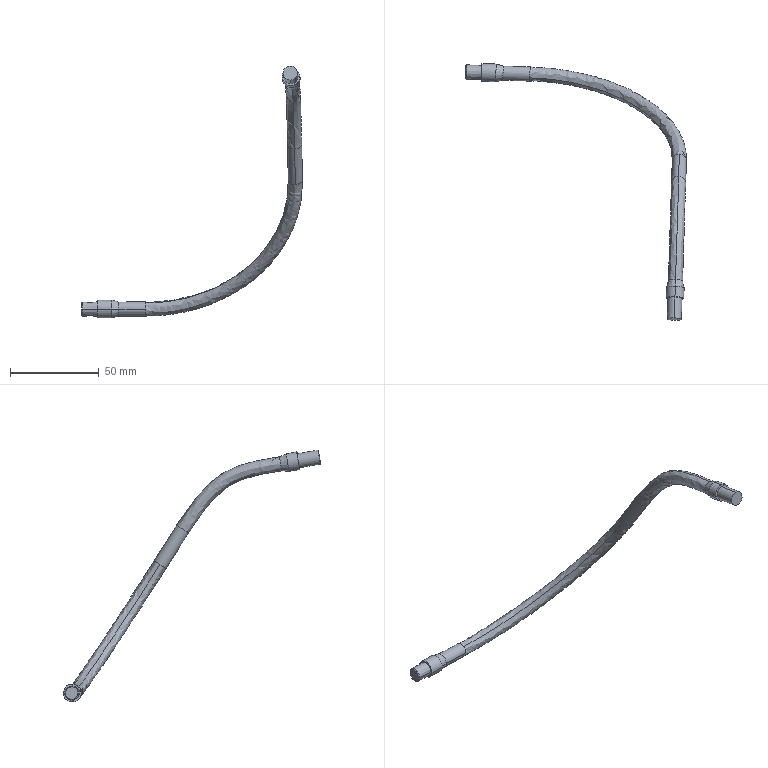Part | SolidWorks | features BaseBody 1 | 1 solid | 26 faces | box 124.46 x 144.887 x 141.873 mm | volume 14890 mm3 | cylinder 10 | cone 8 | spline 4 | plane 4 | commonest cylinder face diameters 8 x6 10 x4